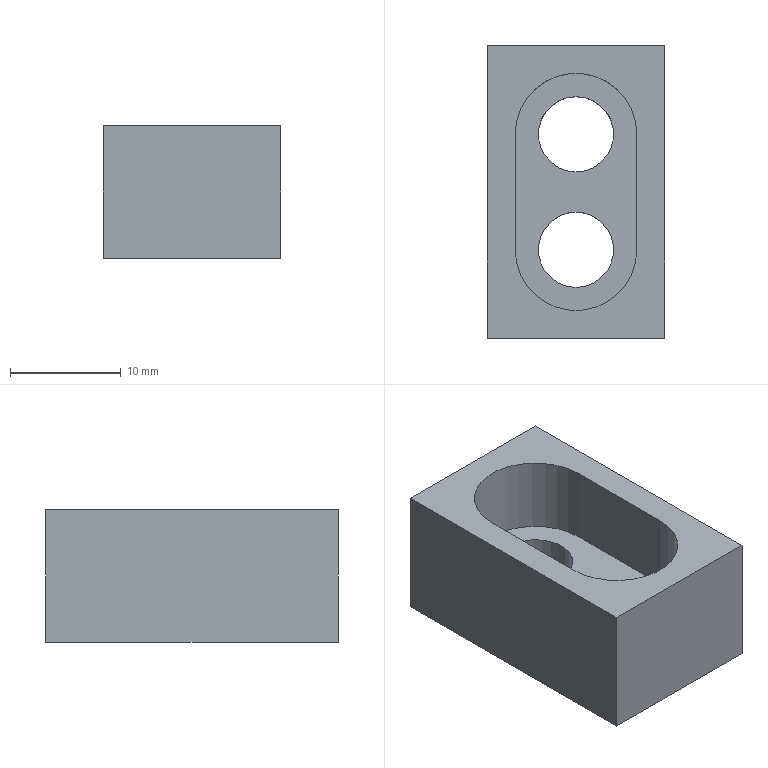Part | NX | features solid 2 | 1 solid | 13 faces | box 16 x 26.434 x 12 mm | volume 3244 mm3 | plane 9 | cylinder 4 | commonest cylinder face diameters 6.8 x2 11 x2
STEP:
#1=CARTESIAN_POINT('',(663.378,-12.569,0.5));
#2=VERTEX_POINT('',#1);
#3=CARTESIAN_POINT('',(663.378,13.865,0.5));
#4=VERTEX_POINT('',#3);
#5=CARTESIAN_POINT('',(663.378,5.865,0.5));
#6=DIRECTION('',(0.,1.,0.));
#7=VECTOR('',#6,1000.);
#8=LINE('',#5,#7);
#9=EDGE_CURVE('',#2,#4,#8,.T.);
#10=ORIENTED_EDGE('',*,*,#9,.F.);
#11=CARTESIAN_POINT('',(679.378,-12.569,0.5));
#12=VERTEX_POINT('',#11);
#13=CARTESIAN_POINT('',(671.378,-12.569,0.5));
#14=DIRECTION('',(1.,0.,0.));
#15=VECTOR('',#14,1000.);
#16=LINE('',#13,#15);
#17=EDGE_CURVE('',#2,#12,#16,.T.);
#18=ORIENTED_EDGE('',*,*,#17,.T.);
#19=CARTESIAN_POINT('',(679.378,13.865,0.5));
#20=VERTEX_POINT('',#19);
#21=CARTESIAN_POINT('',(679.378,5.865,0.5));
#22=DIRECTION('',(0.,-1.,0.));
#23=VECTOR('',#22,1000.);
#24=LINE('',#21,#23);
#25=EDGE_CURVE('',#20,#12,#24,.T.);
#26=ORIENTED_EDGE('',*,*,#25,.F.);
#27=CARTESIAN_POINT('',(671.378,13.865,0.5));
#28=DIRECTION('',(1.,0.,0.));
#29=VECTOR('',#28,1000.);
#30=LINE('',#27,#29);
#31=EDGE_CURVE('',#4,#20,#30,.T.);
#32=ORIENTED_EDGE('',*,*,#31,.F.);
#33=EDGE_LOOP('',(#10,#18,#26,#32));
#34=FACE_BOUND('',#33,.T.);
#35=CARTESIAN_POINT('',(676.878,-4.569,0.5));
#36=VERTEX_POINT('',#35);
#37=CARTESIAN_POINT('',(665.878,-4.569,0.5));
#38=VERTEX_POINT('',#37);
#39=CARTESIAN_POINT('',(671.378,-4.569,0.5));
#40=DIRECTION('',(0.,0.,-1.));
#41=DIRECTION('',(0.,-1.,0.));
#42=AXIS2_PLACEMENT_3D('',#39,#40,#41);
#43=CIRCLE('',#42,5.5);
#44=EDGE_CURVE('',#36,#38,#43,.T.);
#45=ORIENTED_EDGE('',*,*,#44,.T.);
#46=CARTESIAN_POINT('',(665.878,5.865,0.5));
#47=VERTEX_POINT('',#46);
#48=CARTESIAN_POINT('',(665.878,0.648,0.5));
#49=DIRECTION('',(0.,1.,0.));
#50=VECTOR('',#49,1000.);
#51=LINE('',#48,#50);
#52=EDGE_CURVE('',#38,#47,#51,.T.);
#53=ORIENTED_EDGE('',*,*,#52,.T.);
#54=CARTESIAN_POINT('',(676.878,5.865,0.5));
#55=VERTEX_POINT('',#54);
#56=CARTESIAN_POINT('',(671.378,5.865,0.5));
#57=DIRECTION('',(0.,0.,1.));
#58=DIRECTION('',(0.,1.,0.));
#59=AXIS2_PLACEMENT_3D('',#56,#57,#58);
#60=CIRCLE('',#59,5.5);
#61=EDGE_CURVE('',#55,#47,#60,.T.);
#62=ORIENTED_EDGE('',*,*,#61,.F.);
#63=CARTESIAN_POINT('',(676.878,0.648,0.5));
#64=DIRECTION('',(0.,-1.,0.));
#65=VECTOR('',#64,1000.);
#66=LINE('',#63,#65);
#67=EDGE_CURVE('',#55,#36,#66,.T.);
#68=ORIENTED_EDGE('',*,*,#67,.T.);
#69=EDGE_LOOP('',(#45,#53,#62,#68));
#70=FACE_BOUND('',#69,.T.);
#71=CARTESIAN_POINT('',(671.378,5.865,0.5));
#72=DIRECTION('',(0.,0.,1.));
#73=DIRECTION('',(1.,0.,0.));
#74=AXIS2_PLACEMENT_3D('',#71,#72,#73);
#75=PLANE('',#74);
#76=ADVANCED_FACE('',(#34,#70),#75,.T.);
#77=CARTESIAN_POINT('',(665.878,-4.569,-6.5));
#78=VERTEX_POINT('',#77);
#79=CARTESIAN_POINT('',(676.878,-4.569,-6.5));
#80=VERTEX_POINT('',#79);
#81=CARTESIAN_POINT('',(671.378,-4.569,-6.5));
#82=DIRECTION('',(0.,0.,1.));
#83=DIRECTION('',(0.,1.,0.));
#84=AXIS2_PLACEMENT_3D('',#81,#82,#83);
#85=CIRCLE('',#84,5.5);
#86=EDGE_CURVE('',#78,#80,#85,.T.);
#87=ORIENTED_EDGE('',*,*,#86,.F.);
#88=CARTESIAN_POINT('',(665.878,-4.569,-6.5));
#89=DIRECTION('',(0.,0.,1.));
#90=VECTOR('',#89,1000.);
#91=LINE('',#88,#90);
#92=EDGE_CURVE('',#78,#38,#91,.T.);
#93=ORIENTED_EDGE('',*,*,#92,.T.);
#94=ORIENTED_EDGE('',*,*,#44,.F.);
#95=CARTESIAN_POINT('',(676.878,-4.569,-6.5));
#96=DIRECTION('',(0.,0.,-1.));
#97=VECTOR('',#96,1000.);
#98=LINE('',#95,#97);
#99=EDGE_CURVE('',#36,#80,#98,.T.);
#100=ORIENTED_EDGE('',*,*,#99,.T.);
#101=EDGE_LOOP('',(#87,#93,#94,#100));
#102=FACE_BOUND('',#101,.T.);
#103=CARTESIAN_POINT('',(671.378,-4.569,0.5));
#104=DIRECTION('',(0.,0.,-1.));
#105=DIRECTION('',(0.,1.,0.));
#106=AXIS2_PLACEMENT_3D('',#103,#104,#105);
#107=CYLINDRICAL_SURFACE('',#106,5.5);
#108=ADVANCED_FACE('',(#102),#107,.F.);
#109=CARTESIAN_POINT('',(679.378,13.865,-11.5));
#110=VERTEX_POINT('',#109);
#111=CARTESIAN_POINT('',(663.378,13.865,-11.5));
#112=VERTEX_POINT('',#111);
#113=CARTESIAN_POINT('',(671.378,13.865,-11.5));
#114=DIRECTION('',(-1.,0.,0.));
#115=VECTOR('',#114,1000.);
#116=LINE('',#113,#115);
#117=EDGE_CURVE('',#110,#112,#116,.T.);
#118=ORIENTED_EDGE('',*,*,#117,.F.);
#119=CARTESIAN_POINT('',(679.378,-12.569,-11.5));
#120=VERTEX_POINT('',#119);
#121=CARTESIAN_POINT('',(679.378,5.865,-11.5));
#122=DIRECTION('',(0.,1.,0.));
#123=VECTOR('',#122,1000.);
#124=LINE('',#121,#123);
#125=EDGE_CURVE('',#120,#110,#124,.T.);
#126=ORIENTED_EDGE('',*,*,#125,.F.);
#127=CARTESIAN_POINT('',(663.378,-12.569,-11.5));
#128=VERTEX_POINT('',#127);
#129=CARTESIAN_POINT('',(671.378,-12.569,-11.5));
#130=DIRECTION('',(-1.,0.,0.));
#131=VECTOR('',#130,1000.);
#132=LINE('',#129,#131);
#133=EDGE_CURVE('',#120,#128,#132,.T.);
#134=ORIENTED_EDGE('',*,*,#133,.T.);
#135=CARTESIAN_POINT('',(663.378,5.865,-11.5));
#136=DIRECTION('',(0.,-1.,0.));
#137=VECTOR('',#136,1000.);
#138=LINE('',#135,#137);
#139=EDGE_CURVE('',#112,#128,#138,.T.);
#140=ORIENTED_EDGE('',*,*,#139,.F.);
#141=EDGE_LOOP('',(#118,#126,#134,#140));
#142=FACE_BOUND('',#141,.T.);
#143=CARTESIAN_POINT('',(671.378,9.265,-11.5));
#144=VERTEX_POINT('',#143);
#145=CARTESIAN_POINT('',(671.378,5.865,-11.5));
#146=DIRECTION('',(0.,0.,1.));
#147=DIRECTION('',(0.,1.,0.));
#148=AXIS2_PLACEMENT_3D('',#145,#146,#147);
#149=CIRCLE('',#148,3.4);
#150=EDGE_CURVE('',#144,#144,#149,.T.);
#151=ORIENTED_EDGE('',*,*,#150,.T.);
#152=EDGE_LOOP('',(#151));
#153=FACE_BOUND('',#152,.T.);
#154=CARTESIAN_POINT('',(671.378,-7.969,-11.5));
#155=VERTEX_POINT('',#154);
#156=CARTESIAN_POINT('',(671.378,-4.569,-11.5));
#157=DIRECTION('',(0.,0.,-1.));
#158=DIRECTION('',(0.,-1.,0.));
#159=AXIS2_PLACEMENT_3D('',#156,#157,#158);
#160=CIRCLE('',#159,3.4);
#161=EDGE_CURVE('',#155,#155,#160,.T.);
#162=ORIENTED_EDGE('',*,*,#161,.F.);
#163=EDGE_LOOP('',(#162));
#164=FACE_BOUND('',#163,.T.);
#165=CARTESIAN_POINT('',(671.378,5.865,-11.5));
#166=DIRECTION('',(0.,0.,-1.));
#167=DIRECTION('',(-1.,0.,0.));
#168=AXIS2_PLACEMENT_3D('',#165,#166,#167);
#169=PLANE('',#168);
#170=ADVANCED_FACE('',(#142,#153,#164),#169,.T.);
#171=ORIENTED_EDGE('',*,*,#25,.T.);
#172=CARTESIAN_POINT('',(679.378,-12.569,0.5));
#173=DIRECTION('',(0.,0.,-1.));
#174=VECTOR('',#173,1000.);
#175=LINE('',#172,#174);
#176=EDGE_CURVE('',#12,#120,#175,.T.);
#177=ORIENTED_EDGE('',*,*,#176,.T.);
#178=ORIENTED_EDGE('',*,*,#125,.T.);
#179=CARTESIAN_POINT('',(679.378,13.865,0.5));
#180=DIRECTION('',(0.,0.,-1.));
#181=VECTOR('',#180,1000.);
#182=LINE('',#179,#181);
#183=EDGE_CURVE('',#20,#110,#182,.T.);
#184=ORIENTED_EDGE('',*,*,#183,.F.);
#185=EDGE_LOOP('',(#171,#177,#178,#184));
#186=FACE_BOUND('',#185,.T.);
#187=CARTESIAN_POINT('',(679.378,5.865,0.5));
#188=DIRECTION('',(1.,0.,0.));
#189=DIRECTION('',(0.,0.,-1.));
#190=AXIS2_PLACEMENT_3D('',#187,#188,#189);
#191=PLANE('',#190);
#192=ADVANCED_FACE('',(#186),#191,.T.);
#193=ORIENTED_EDGE('',*,*,#139,.T.);
#194=CARTESIAN_POINT('',(663.378,-12.569,0.5));
#195=DIRECTION('',(0.,0.,-1.));
#196=VECTOR('',#195,1000.);
#197=LINE('',#194,#196);
#198=EDGE_CURVE('',#2,#128,#197,.T.);
#199=ORIENTED_EDGE('',*,*,#198,.F.);
#200=ORIENTED_EDGE('',*,*,#9,.T.);
#201=CARTESIAN_POINT('',(663.378,13.865,0.5));
#202=DIRECTION('',(0.,0.,-1.));
#203=VECTOR('',#202,1000.);
#204=LINE('',#201,#203);
#205=EDGE_CURVE('',#4,#112,#204,.T.);
#206=ORIENTED_EDGE('',*,*,#205,.T.);
#207=EDGE_LOOP('',(#193,#199,#200,#206));
#208=FACE_BOUND('',#207,.T.);
#209=CARTESIAN_POINT('',(663.378,5.865,0.5));
#210=DIRECTION('',(-1.,0.,0.));
#211=DIRECTION('',(0.,0.,1.));
#212=AXIS2_PLACEMENT_3D('',#209,#210,#211);
#213=PLANE('',#212);
#214=ADVANCED_FACE('',(#208),#213,.T.);
#215=ORIENTED_EDGE('',*,*,#183,.T.);
#216=ORIENTED_EDGE('',*,*,#117,.T.);
#217=ORIENTED_EDGE('',*,*,#205,.F.);
#218=ORIENTED_EDGE('',*,*,#31,.T.);
#219=EDGE_LOOP('',(#215,#216,#217,#218));
#220=FACE_BOUND('',#219,.T.);
#221=CARTESIAN_POINT('',(671.378,13.865,0.5));
#222=DIRECTION('',(0.,1.,0.));
#223=DIRECTION('',(0.,0.,-1.));
#224=AXIS2_PLACEMENT_3D('',#221,#222,#223);
#225=PLANE('',#224);
#226=ADVANCED_FACE('',(#220),#225,.T.);
#227=CARTESIAN_POINT('',(671.378,2.465,-6.5));
#228=VERTEX_POINT('',#227);
#229=CARTESIAN_POINT('',(671.378,5.865,-6.5));
#230=DIRECTION('',(0.,0.,-1.));
#231=DIRECTION('',(0.,-1.,0.));
#232=AXIS2_PLACEMENT_3D('',#229,#230,#231);
#233=CIRCLE('',#232,3.4);
#234=EDGE_CURVE('',#228,#228,#233,.T.);
#235=ORIENTED_EDGE('',*,*,#234,.F.);
#236=EDGE_LOOP('',(#235));
#237=FACE_BOUND('',#236,.T.);
#238=ORIENTED_EDGE('',*,*,#150,.F.);
#239=EDGE_LOOP('',(#238));
#240=FACE_BOUND('',#239,.T.);
#241=CARTESIAN_POINT('',(671.378,5.865,-49.5));
#242=DIRECTION('',(0.,0.,-1.));
#243=DIRECTION('',(0.,-1.,0.));
#244=AXIS2_PLACEMENT_3D('',#241,#242,#243);
#245=CYLINDRICAL_SURFACE('',#244,3.4);
#246=ADVANCED_FACE('',(#237,#240),#245,.F.);
#247=ORIENTED_EDGE('',*,*,#234,.T.);
#248=EDGE_LOOP('',(#247));
#249=FACE_BOUND('',#248,.T.);
#250=CARTESIAN_POINT('',(676.878,5.865,-6.5));
#251=VERTEX_POINT('',#250);
#252=CARTESIAN_POINT('',(665.878,5.865,-6.5));
#253=VERTEX_POINT('',#252);
#254=CARTESIAN_POINT('',(671.378,5.865,-6.5));
#255=DIRECTION('',(0.,0.,-1.));
#256=DIRECTION('',(0.,-1.,0.));
#257=AXIS2_PLACEMENT_3D('',#254,#255,#256);
#258=CIRCLE('',#257,5.5);
#259=EDGE_CURVE('',#251,#253,#258,.F.);
#260=ORIENTED_EDGE('',*,*,#259,.T.);
#261=CARTESIAN_POINT('',(665.878,0.648,-6.5));
#262=DIRECTION('',(0.,-1.,0.));
#263=VECTOR('',#262,1000.);
#264=LINE('',#261,#263);
#265=EDGE_CURVE('',#253,#78,#264,.T.);
#266=ORIENTED_EDGE('',*,*,#265,.T.);
#267=ORIENTED_EDGE('',*,*,#86,.T.);
#268=CARTESIAN_POINT('',(676.878,0.648,-6.5));
#269=DIRECTION('',(0.,1.,0.));
#270=VECTOR('',#269,1000.);
#271=LINE('',#268,#270);
#272=EDGE_CURVE('',#80,#251,#271,.T.);
#273=ORIENTED_EDGE('',*,*,#272,.T.);
#274=EDGE_LOOP('',(#260,#266,#267,#273));
#275=FACE_BOUND('',#274,.T.);
#276=CARTESIAN_POINT('',(671.378,-1.169,-6.5));
#277=VERTEX_POINT('',#276);
#278=CARTESIAN_POINT('',(671.378,-4.569,-6.5));
#279=DIRECTION('',(0.,0.,1.));
#280=DIRECTION('',(0.,1.,0.));
#281=AXIS2_PLACEMENT_3D('',#278,#279,#280);
#282=CIRCLE('',#281,3.4);
#283=EDGE_CURVE('',#277,#277,#282,.T.);
#284=ORIENTED_EDGE('',*,*,#283,.F.);
#285=EDGE_LOOP('',(#284));
#286=FACE_BOUND('',#285,.T.);
#287=CARTESIAN_POINT('',(671.378,5.865,-6.5));
#288=DIRECTION('',(0.,0.,1.));
#289=DIRECTION('',(1.,0.,0.));
#290=AXIS2_PLACEMENT_3D('',#287,#288,#289);
#291=PLANE('',#290);
#292=ADVANCED_FACE('',(#249,#275,#286),#291,.T.);
#293=ORIENTED_EDGE('',*,*,#259,.F.);
#294=CARTESIAN_POINT('',(676.878,5.865,-6.5));
#295=DIRECTION('',(0.,0.,1.));
#296=VECTOR('',#295,1000.);
#297=LINE('',#294,#296);
#298=EDGE_CURVE('',#251,#55,#297,.T.);
#299=ORIENTED_EDGE('',*,*,#298,.T.);
#300=ORIENTED_EDGE('',*,*,#61,.T.);
#301=CARTESIAN_POINT('',(665.878,5.865,-6.5));
#302=DIRECTION('',(0.,0.,-1.));
#303=VECTOR('',#302,1000.);
#304=LINE('',#301,#303);
#305=EDGE_CURVE('',#47,#253,#304,.T.);
#306=ORIENTED_EDGE('',*,*,#305,.T.);
#307=EDGE_LOOP('',(#293,#299,#300,#306));
#308=FACE_BOUND('',#307,.T.);
#309=CARTESIAN_POINT('',(671.378,5.865,0.5));
#310=DIRECTION('',(0.,0.,-1.));
#311=DIRECTION('',(0.,-1.,0.));
#312=AXIS2_PLACEMENT_3D('',#309,#310,#311);
#313=CYLINDRICAL_SURFACE('',#312,5.5);
#314=ADVANCED_FACE('',(#308),#313,.F.);
#315=ORIENTED_EDGE('',*,*,#176,.F.);
#316=ORIENTED_EDGE('',*,*,#17,.F.);
#317=ORIENTED_EDGE('',*,*,#198,.T.);
#318=ORIENTED_EDGE('',*,*,#133,.F.);
#319=EDGE_LOOP('',(#315,#316,#317,#318));
#320=FACE_BOUND('',#319,.T.);
#321=CARTESIAN_POINT('',(671.378,-12.569,0.5));
#322=DIRECTION('',(0.,-1.,0.));
#323=DIRECTION('',(0.,0.,-1.));
#324=AXIS2_PLACEMENT_3D('',#321,#322,#323);
#325=PLANE('',#324);
#326=ADVANCED_FACE('',(#320),#325,.T.);
#327=ORIENTED_EDGE('',*,*,#283,.T.);
#328=EDGE_LOOP('',(#327));
#329=FACE_BOUND('',#328,.T.);
#330=ORIENTED_EDGE('',*,*,#161,.T.);
#331=EDGE_LOOP('',(#330));
#332=FACE_BOUND('',#331,.T.);
#333=CARTESIAN_POINT('',(671.378,-4.569,-49.5));
#334=DIRECTION('',(0.,0.,-1.));
#335=DIRECTION('',(0.,1.,0.));
#336=AXIS2_PLACEMENT_3D('',#333,#334,#335);
#337=CYLINDRICAL_SURFACE('',#336,3.4);
#338=ADVANCED_FACE('',(#329,#332),#337,.F.);
#339=ORIENTED_EDGE('',*,*,#265,.F.);
#340=ORIENTED_EDGE('',*,*,#305,.F.);
#341=ORIENTED_EDGE('',*,*,#52,.F.);
#342=ORIENTED_EDGE('',*,*,#92,.F.);
#343=EDGE_LOOP('',(#339,#340,#341,#342));
#344=FACE_BOUND('',#343,.T.);
#345=CARTESIAN_POINT('',(665.878,0.648,-6.5));
#346=DIRECTION('',(-1.,0.,0.));
#347=DIRECTION('',(0.,0.,1.));
#348=AXIS2_PLACEMENT_3D('',#345,#346,#347);
#349=PLANE('',#348);
#350=ADVANCED_FACE('',(#344),#349,.F.);
#351=ORIENTED_EDGE('',*,*,#67,.F.);
#352=ORIENTED_EDGE('',*,*,#298,.F.);
#353=ORIENTED_EDGE('',*,*,#272,.F.);
#354=ORIENTED_EDGE('',*,*,#99,.F.);
#355=EDGE_LOOP('',(#351,#352,#353,#354));
#356=FACE_BOUND('',#355,.T.);
#357=CARTESIAN_POINT('',(676.878,0.648,-6.5));
#358=DIRECTION('',(1.,0.,0.));
#359=DIRECTION('',(0.,0.,-1.));
#360=AXIS2_PLACEMENT_3D('',#357,#358,#359);
#361=PLANE('',#360);
#362=ADVANCED_FACE('',(#356),#361,.F.);
#363=CLOSED_SHELL('',(#76,#108,#170,#192,#214,#226,#246,#292,#314,#326,#338,#350,#362));
#364=MANIFOLD_SOLID_BREP('',#363);
#365=(LENGTH_UNIT()NAMED_UNIT(*)SI_UNIT(.MILLI.,.METRE.));
#366=UNCERTAINTY_MEASURE_WITH_UNIT(LENGTH_MEASURE(0.00001),#365,'','');
#367=(NAMED_UNIT(*)PLANE_ANGLE_UNIT()SI_UNIT($,.RADIAN.));
#368=(NAMED_UNIT(*)SI_UNIT($,.STERADIAN.)SOLID_ANGLE_UNIT());
#369=(GEOMETRIC_REPRESENTATION_CONTEXT(3)GLOBAL_UNCERTAINTY_ASSIGNED_CONTEXT((#366))GLOBAL_UNIT_ASSIGNED_CONTEXT((#365,#367,#368))REPRESENTATION_CONTEXT('',''));
#370=ADVANCED_BREP_SHAPE_REPRESENTATION('',(#364),#369);